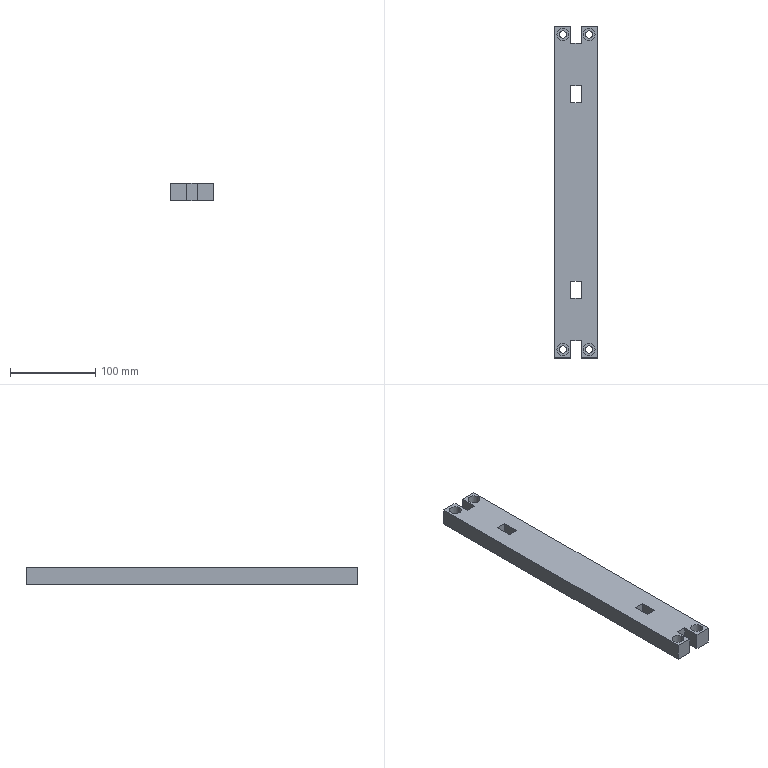Part | STEP file | 冲床-300配套压波_id178_x_t | 1 solid | 34 faces | box 50 x 390 x 20 mm | volume 362265 mm3 | plane 26 | cylinder 8 | commonest cylinder face diameters 8.7 x4 14 x4
STEP:
#1=CARTESIAN_POINT('',(1118.85,-185.,60.));
#2=VERTEX_POINT('',#1);
#3=CARTESIAN_POINT('',(1114.5,-185.,60.));
#4=DIRECTION('',(0.,0.,1.));
#5=DIRECTION('',(1.,0.,0.));
#6=AXIS2_PLACEMENT_3D('',#3,#4,#5);
#7=CIRCLE('',#6,4.35);
#8=EDGE_CURVE('',#2,#2,#7,.T.);
#9=ORIENTED_EDGE('',*,*,#8,.F.);
#10=EDGE_LOOP('',(#9));
#11=FACE_BOUND('',#10,.T.);
#12=CARTESIAN_POINT('',(1121.5,-185.,60.));
#13=VERTEX_POINT('',#12);
#14=CARTESIAN_POINT('',(1114.5,-185.,60.));
#15=DIRECTION('',(0.,0.,1.));
#16=DIRECTION('',(1.,0.,0.));
#17=AXIS2_PLACEMENT_3D('',#14,#15,#16);
#18=CIRCLE('',#17,7.);
#19=EDGE_CURVE('',#13,#13,#18,.T.);
#20=ORIENTED_EDGE('',*,*,#19,.T.);
#21=EDGE_LOOP('',(#20));
#22=FACE_BOUND('',#21,.T.);
#23=CARTESIAN_POINT('',(1114.5,-185.,60.));
#24=DIRECTION('',(0.,0.,-1.));
#25=DIRECTION('',(1.,0.,0.));
#26=AXIS2_PLACEMENT_3D('',#23,#24,#25);
#27=PLANE('',#26);
#28=ADVANCED_FACE('',(#11,#22),#27,.F.);
#29=CARTESIAN_POINT('',(1118.85,-185.,50.));
#30=VERTEX_POINT('',#29);
#31=CARTESIAN_POINT('',(1114.5,-185.,50.));
#32=DIRECTION('',(0.,0.,-1.));
#33=DIRECTION('',(1.,0.,0.));
#34=AXIS2_PLACEMENT_3D('',#31,#32,#33);
#35=CIRCLE('',#34,4.35);
#36=EDGE_CURVE('',#30,#30,#35,.T.);
#37=ORIENTED_EDGE('',*,*,#36,.T.);
#38=EDGE_LOOP('',(#37));
#39=FACE_BOUND('',#38,.T.);
#40=ORIENTED_EDGE('',*,*,#8,.T.);
#41=EDGE_LOOP('',(#40));
#42=FACE_BOUND('',#41,.T.);
#43=CARTESIAN_POINT('',(1114.5,-185.,-46.884));
#44=DIRECTION('',(0.,0.,-1.));
#45=DIRECTION('',(1.,0.,0.));
#46=AXIS2_PLACEMENT_3D('',#43,#44,#45);
#47=CYLINDRICAL_SURFACE('',#46,4.35);
#48=ADVANCED_FACE('',(#39,#42),#47,.F.);
#49=ORIENTED_EDGE('',*,*,#19,.F.);
#50=EDGE_LOOP('',(#49));
#51=FACE_BOUND('',#50,.T.);
#52=CARTESIAN_POINT('',(1121.5,-185.,70.));
#53=VERTEX_POINT('',#52);
#54=CARTESIAN_POINT('',(1114.5,-185.,70.));
#55=DIRECTION('',(0.,0.,1.));
#56=DIRECTION('',(1.,0.,0.));
#57=AXIS2_PLACEMENT_3D('',#54,#55,#56);
#58=CIRCLE('',#57,7.);
#59=EDGE_CURVE('',#53,#53,#58,.T.);
#60=ORIENTED_EDGE('',*,*,#59,.T.);
#61=EDGE_LOOP('',(#60));
#62=FACE_BOUND('',#61,.T.);
#63=CARTESIAN_POINT('',(1114.5,-185.,70.));
#64=DIRECTION('',(0.,0.,-1.));
#65=DIRECTION('',(1.,0.,0.));
#66=AXIS2_PLACEMENT_3D('',#63,#64,#65);
#67=CYLINDRICAL_SURFACE('',#66,7.);
#68=ADVANCED_FACE('',(#51,#62),#67,.F.);
#69=CARTESIAN_POINT('',(1141.15,-185.,60.));
#70=VERTEX_POINT('',#69);
#71=CARTESIAN_POINT('',(1145.5,-185.,60.));
#72=DIRECTION('',(0.,0.,1.));
#73=DIRECTION('',(-1.,0.,0.));
#74=AXIS2_PLACEMENT_3D('',#71,#72,#73);
#75=CIRCLE('',#74,4.35);
#76=EDGE_CURVE('',#70,#70,#75,.T.);
#77=ORIENTED_EDGE('',*,*,#76,.F.);
#78=EDGE_LOOP('',(#77));
#79=FACE_BOUND('',#78,.T.);
#80=CARTESIAN_POINT('',(1138.5,-185.,60.));
#81=VERTEX_POINT('',#80);
#82=CARTESIAN_POINT('',(1145.5,-185.,60.));
#83=DIRECTION('',(0.,0.,1.));
#84=DIRECTION('',(-1.,0.,0.));
#85=AXIS2_PLACEMENT_3D('',#82,#83,#84);
#86=CIRCLE('',#85,7.);
#87=EDGE_CURVE('',#81,#81,#86,.T.);
#88=ORIENTED_EDGE('',*,*,#87,.T.);
#89=EDGE_LOOP('',(#88));
#90=FACE_BOUND('',#89,.T.);
#91=CARTESIAN_POINT('',(1145.5,-185.,60.));
#92=DIRECTION('',(0.,0.,-1.));
#93=DIRECTION('',(-1.,0.,0.));
#94=AXIS2_PLACEMENT_3D('',#91,#92,#93);
#95=PLANE('',#94);
#96=ADVANCED_FACE('',(#79,#90),#95,.F.);
#97=CARTESIAN_POINT('',(1136.,-105.,70.));
#98=VERTEX_POINT('',#97);
#99=CARTESIAN_POINT('',(1136.,-125.,70.));
#100=VERTEX_POINT('',#99);
#101=CARTESIAN_POINT('',(1136.,-105.,70.));
#102=DIRECTION('',(0.,-1.,0.));
#103=VECTOR('',#102,1.);
#104=LINE('',#101,#103);
#105=EDGE_CURVE('',#98,#100,#104,.T.);
#106=ORIENTED_EDGE('',*,*,#105,.F.);
#107=CARTESIAN_POINT('',(1136.,-105.,50.));
#108=VERTEX_POINT('',#107);
#109=CARTESIAN_POINT('',(1136.,-105.,150.));
#110=DIRECTION('',(0.,0.,1.));
#111=VECTOR('',#110,1.);
#112=LINE('',#109,#111);
#113=EDGE_CURVE('',#108,#98,#112,.T.);
#114=ORIENTED_EDGE('',*,*,#113,.F.);
#115=CARTESIAN_POINT('',(1136.,-125.,50.));
#116=VERTEX_POINT('',#115);
#117=CARTESIAN_POINT('',(1136.,-125.,50.));
#118=DIRECTION('',(0.,-1.,0.));
#119=VECTOR('',#118,1.);
#120=LINE('',#117,#119);
#121=EDGE_CURVE('',#108,#116,#120,.T.);
#122=ORIENTED_EDGE('',*,*,#121,.T.);
#123=CARTESIAN_POINT('',(1136.,-125.,46.));
#124=DIRECTION('',(0.,0.,-1.));
#125=VECTOR('',#124,1.);
#126=LINE('',#123,#125);
#127=EDGE_CURVE('',#100,#116,#126,.T.);
#128=ORIENTED_EDGE('',*,*,#127,.F.);
#129=EDGE_LOOP('',(#106,#114,#122,#128));
#130=FACE_OUTER_BOUND('',#129,.T.);
#131=CARTESIAN_POINT('',(1136.,-125.,46.));
#132=DIRECTION('',(1.,0.,0.));
#133=DIRECTION('',(0.,0.,-1.));
#134=AXIS2_PLACEMENT_3D('',#131,#132,#133);
#135=PLANE('',#134);
#136=ADVANCED_FACE('',(#130),#135,.F.);
#137=ORIENTED_EDGE('',*,*,#113,.T.);
#138=CARTESIAN_POINT('',(1124.,-105.,70.));
#139=VERTEX_POINT('',#138);
#140=CARTESIAN_POINT('',(1105.,-105.,70.));
#141=DIRECTION('',(-1.,0.,0.));
#142=VECTOR('',#141,1.);
#143=LINE('',#140,#142);
#144=EDGE_CURVE('',#98,#139,#143,.T.);
#145=ORIENTED_EDGE('',*,*,#144,.T.);
#146=CARTESIAN_POINT('',(1124.,-105.,50.));
#147=VERTEX_POINT('',#146);
#148=CARTESIAN_POINT('',(1124.,-105.,150.));
#149=DIRECTION('',(0.,0.,-1.));
#150=VECTOR('',#149,1.);
#151=LINE('',#148,#150);
#152=EDGE_CURVE('',#139,#147,#151,.T.);
#153=ORIENTED_EDGE('',*,*,#152,.T.);
#154=CARTESIAN_POINT('',(1105.,-105.,50.));
#155=DIRECTION('',(-1.,0.,0.));
#156=VECTOR('',#155,1.);
#157=LINE('',#154,#156);
#158=EDGE_CURVE('',#108,#147,#157,.T.);
#159=ORIENTED_EDGE('',*,*,#158,.F.);
#160=EDGE_LOOP('',(#137,#145,#153,#159));
#161=FACE_OUTER_BOUND('',#160,.T.);
#162=CARTESIAN_POINT('',(1105.,-105.,150.));
#163=DIRECTION('',(0.,-1.,0.));
#164=DIRECTION('',(0.,0.,1.));
#165=AXIS2_PLACEMENT_3D('',#162,#163,#164);
#166=PLANE('',#165);
#167=ADVANCED_FACE('',(#161),#166,.T.);
#168=ORIENTED_EDGE('',*,*,#152,.F.);
#169=CARTESIAN_POINT('',(1124.,-125.,70.));
#170=VERTEX_POINT('',#169);
#171=CARTESIAN_POINT('',(1124.,-105.,70.));
#172=DIRECTION('',(0.,1.,0.));
#173=VECTOR('',#172,1.);
#174=LINE('',#171,#173);
#175=EDGE_CURVE('',#170,#139,#174,.T.);
#176=ORIENTED_EDGE('',*,*,#175,.F.);
#177=CARTESIAN_POINT('',(1124.,-125.,50.));
#178=VERTEX_POINT('',#177);
#179=CARTESIAN_POINT('',(1124.,-125.,78.));
#180=DIRECTION('',(0.,0.,1.));
#181=VECTOR('',#180,1.);
#182=LINE('',#179,#181);
#183=EDGE_CURVE('',#178,#170,#182,.T.);
#184=ORIENTED_EDGE('',*,*,#183,.F.);
#185=CARTESIAN_POINT('',(1124.,-105.,50.));
#186=DIRECTION('',(0.,-1.,0.));
#187=VECTOR('',#186,1.);
#188=LINE('',#185,#187);
#189=EDGE_CURVE('',#147,#178,#188,.T.);
#190=ORIENTED_EDGE('',*,*,#189,.F.);
#191=EDGE_LOOP('',(#168,#176,#184,#190));
#192=FACE_OUTER_BOUND('',#191,.T.);
#193=CARTESIAN_POINT('',(1124.,-125.,78.));
#194=DIRECTION('',(-1.,0.,0.));
#195=DIRECTION('',(0.,0.,1.));
#196=AXIS2_PLACEMENT_3D('',#193,#194,#195);
#197=PLANE('',#196);
#198=ADVANCED_FACE('',(#192),#197,.F.);
#199=ORIENTED_EDGE('',*,*,#183,.T.);
#200=CARTESIAN_POINT('',(1105.,-125.,70.));
#201=DIRECTION('',(1.,0.,0.));
#202=VECTOR('',#201,1.);
#203=LINE('',#200,#202);
#204=EDGE_CURVE('',#170,#100,#203,.T.);
#205=ORIENTED_EDGE('',*,*,#204,.T.);
#206=ORIENTED_EDGE('',*,*,#127,.T.);
#207=CARTESIAN_POINT('',(1155.,-125.,50.));
#208=DIRECTION('',(-1.,0.,0.));
#209=VECTOR('',#208,1.);
#210=LINE('',#207,#209);
#211=EDGE_CURVE('',#116,#178,#210,.T.);
#212=ORIENTED_EDGE('',*,*,#211,.T.);
#213=EDGE_LOOP('',(#199,#205,#206,#212));
#214=FACE_OUTER_BOUND('',#213,.T.);
#215=CARTESIAN_POINT('',(1155.,-125.,150.));
#216=DIRECTION('',(0.,1.,0.));
#217=DIRECTION('',(0.,0.,-1.));
#218=AXIS2_PLACEMENT_3D('',#215,#216,#217);
#219=PLANE('',#218);
#220=ADVANCED_FACE('',(#214),#219,.T.);
#221=CARTESIAN_POINT('',(1155.,-195.,50.));
#222=VERTEX_POINT('',#221);
#223=CARTESIAN_POINT('',(1155.,195.,50.));
#224=VERTEX_POINT('',#223);
#225=CARTESIAN_POINT('',(1155.,-105.,50.));
#226=DIRECTION('',(0.,1.,0.));
#227=VECTOR('',#226,1.);
#228=LINE('',#225,#227);
#229=EDGE_CURVE('',#222,#224,#228,.T.);
#230=ORIENTED_EDGE('',*,*,#229,.T.);
#231=CARTESIAN_POINT('',(1155.,195.,70.));
#232=VERTEX_POINT('',#231);
#233=CARTESIAN_POINT('',(1155.,195.,50.));
#234=DIRECTION('',(0.,0.,-1.));
#235=VECTOR('',#234,1.);
#236=LINE('',#233,#235);
#237=EDGE_CURVE('',#232,#224,#236,.T.);
#238=ORIENTED_EDGE('',*,*,#237,.F.);
#239=CARTESIAN_POINT('',(1155.,-195.,70.));
#240=VERTEX_POINT('',#239);
#241=CARTESIAN_POINT('',(1155.,-105.,70.));
#242=DIRECTION('',(0.,1.,0.));
#243=VECTOR('',#242,1.);
#244=LINE('',#241,#243);
#245=EDGE_CURVE('',#240,#232,#244,.T.);
#246=ORIENTED_EDGE('',*,*,#245,.F.);
#247=CARTESIAN_POINT('',(1155.,-195.,50.));
#248=DIRECTION('',(0.,0.,-1.));
#249=VECTOR('',#248,1.);
#250=LINE('',#247,#249);
#251=EDGE_CURVE('',#240,#222,#250,.T.);
#252=ORIENTED_EDGE('',*,*,#251,.T.);
#253=EDGE_LOOP('',(#230,#238,#246,#252));
#254=FACE_OUTER_BOUND('',#253,.T.);
#255=CARTESIAN_POINT('',(1155.,-105.,70.));
#256=DIRECTION('',(1.,0.,0.));
#257=DIRECTION('',(0.,0.,-1.));
#258=AXIS2_PLACEMENT_3D('',#255,#256,#257);
#259=PLANE('',#258);
#260=ADVANCED_FACE('',(#254),#259,.T.);
#261=CARTESIAN_POINT('',(1136.,-195.,50.));
#262=VERTEX_POINT('',#261);
#263=CARTESIAN_POINT('',(1136.,-195.,70.));
#264=VERTEX_POINT('',#263);
#265=CARTESIAN_POINT('',(1136.,-195.,70.));
#266=DIRECTION('',(0.,0.,1.));
#267=VECTOR('',#266,1.);
#268=LINE('',#265,#267);
#269=EDGE_CURVE('',#262,#264,#268,.T.);
#270=ORIENTED_EDGE('',*,*,#269,.F.);
#271=CARTESIAN_POINT('',(1155.,-195.,50.));
#272=DIRECTION('',(-1.,0.,0.));
#273=VECTOR('',#272,1.);
#274=LINE('',#271,#273);
#275=EDGE_CURVE('',#222,#262,#274,.T.);
#276=ORIENTED_EDGE('',*,*,#275,.F.);
#277=ORIENTED_EDGE('',*,*,#251,.F.);
#278=CARTESIAN_POINT('',(1155.,-195.,70.));
#279=DIRECTION('',(1.,0.,0.));
#280=VECTOR('',#279,1.);
#281=LINE('',#278,#280);
#282=EDGE_CURVE('',#264,#240,#281,.T.);
#283=ORIENTED_EDGE('',*,*,#282,.F.);
#284=EDGE_LOOP('',(#270,#276,#277,#283));
#285=FACE_OUTER_BOUND('',#284,.T.);
#286=CARTESIAN_POINT('',(1155.,-195.,50.));
#287=DIRECTION('',(0.,1.,0.));
#288=DIRECTION('',(0.,0.,-1.));
#289=AXIS2_PLACEMENT_3D('',#286,#287,#288);
#290=PLANE('',#289);
#291=ADVANCED_FACE('',(#285),#290,.F.);
#292=ORIENTED_EDGE('',*,*,#269,.T.);
#293=CARTESIAN_POINT('',(1136.,-175.,70.));
#294=VERTEX_POINT('',#293);
#295=CARTESIAN_POINT('',(1136.,-175.,70.));
#296=DIRECTION('',(0.,-1.,0.));
#297=VECTOR('',#296,1.);
#298=LINE('',#295,#297);
#299=EDGE_CURVE('',#294,#264,#298,.T.);
#300=ORIENTED_EDGE('',*,*,#299,.F.);
#301=CARTESIAN_POINT('',(1136.,-175.,50.));
#302=VERTEX_POINT('',#301);
#303=CARTESIAN_POINT('',(1136.,-175.,70.));
#304=DIRECTION('',(0.,0.,-1.));
#305=VECTOR('',#304,1.);
#306=LINE('',#303,#305);
#307=EDGE_CURVE('',#294,#302,#306,.T.);
#308=ORIENTED_EDGE('',*,*,#307,.T.);
#309=CARTESIAN_POINT('',(1136.,-175.,50.));
#310=DIRECTION('',(0.,-1.,0.));
#311=VECTOR('',#310,1.);
#312=LINE('',#309,#311);
#313=EDGE_CURVE('',#302,#262,#312,.T.);
#314=ORIENTED_EDGE('',*,*,#313,.T.);
#315=EDGE_LOOP('',(#292,#300,#308,#314));
#316=FACE_OUTER_BOUND('',#315,.T.);
#317=CARTESIAN_POINT('',(1136.,-175.,70.));
#318=DIRECTION('',(1.,0.,0.));
#319=DIRECTION('',(0.,0.,-1.));
#320=AXIS2_PLACEMENT_3D('',#317,#318,#319);
#321=PLANE('',#320);
#322=ADVANCED_FACE('',(#316),#321,.F.);
#323=CARTESIAN_POINT('',(1124.,-175.,50.));
#324=VERTEX_POINT('',#323);
#325=CARTESIAN_POINT('',(1155.,-175.,50.));
#326=DIRECTION('',(-1.,0.,0.));
#327=VECTOR('',#326,1.);
#328=LINE('',#325,#327);
#329=EDGE_CURVE('',#302,#324,#328,.T.);
#330=ORIENTED_EDGE('',*,*,#329,.F.);
#331=ORIENTED_EDGE('',*,*,#307,.F.);
#332=CARTESIAN_POINT('',(1124.,-175.,70.));
#333=VERTEX_POINT('',#332);
#334=CARTESIAN_POINT('',(1124.,-175.,70.));
#335=DIRECTION('',(1.,0.,0.));
#336=VECTOR('',#335,1.);
#337=LINE('',#334,#336);
#338=EDGE_CURVE('',#333,#294,#337,.T.);
#339=ORIENTED_EDGE('',*,*,#338,.F.);
#340=CARTESIAN_POINT('',(1124.,-175.,50.));
#341=DIRECTION('',(0.,0.,1.));
#342=VECTOR('',#341,1.);
#343=LINE('',#340,#342);
#344=EDGE_CURVE('',#324,#333,#343,.T.);
#345=ORIENTED_EDGE('',*,*,#344,.F.);
#346=EDGE_LOOP('',(#330,#331,#339,#345));
#347=FACE_OUTER_BOUND('',#346,.T.);
#348=CARTESIAN_POINT('',(1155.,-175.,50.));
#349=DIRECTION('',(0.,1.,0.));
#350=DIRECTION('',(0.,0.,-1.));
#351=AXIS2_PLACEMENT_3D('',#348,#349,#350);
#352=PLANE('',#351);
#353=ADVANCED_FACE('',(#347),#352,.F.);
#354=CARTESIAN_POINT('',(1124.,-195.,70.));
#355=VERTEX_POINT('',#354);
#356=CARTESIAN_POINT('',(1124.,-195.,50.));
#357=VERTEX_POINT('',#356);
#358=CARTESIAN_POINT('',(1124.,-195.,50.));
#359=DIRECTION('',(0.,0.,-1.));
#360=VECTOR('',#359,1.);
#361=LINE('',#358,#360);
#362=EDGE_CURVE('',#355,#357,#361,.T.);
#363=ORIENTED_EDGE('',*,*,#362,.T.);
#364=CARTESIAN_POINT('',(1124.,-175.,50.));
#365=DIRECTION('',(0.,-1.,0.));
#366=VECTOR('',#365,1.);
#367=LINE('',#364,#366);
#368=EDGE_CURVE('',#324,#357,#367,.T.);
#369=ORIENTED_EDGE('',*,*,#368,.F.);
#370=ORIENTED_EDGE('',*,*,#344,.T.);
#371=CARTESIAN_POINT('',(1124.,-175.,70.));
#372=DIRECTION('',(0.,-1.,0.));
#373=VECTOR('',#372,1.);
#374=LINE('',#371,#373);
#375=EDGE_CURVE('',#333,#355,#374,.T.);
#376=ORIENTED_EDGE('',*,*,#375,.T.);
#377=EDGE_LOOP('',(#363,#369,#370,#376));
#378=FACE_OUTER_BOUND('',#377,.T.);
#379=CARTESIAN_POINT('',(1124.,-175.,50.));
#380=DIRECTION('',(-1.,0.,0.));
#381=DIRECTION('',(0.,0.,1.));
#382=AXIS2_PLACEMENT_3D('',#379,#380,#381);
#383=PLANE('',#382);
#384=ADVANCED_FACE('',(#378),#383,.F.);
#385=ORIENTED_EDGE('',*,*,#362,.F.);
#386=CARTESIAN_POINT('',(1105.,-195.,70.));
#387=VERTEX_POINT('',#386);
#388=CARTESIAN_POINT('',(1155.,-195.,70.));
#389=DIRECTION('',(1.,0.,0.));
#390=VECTOR('',#389,1.);
#391=LINE('',#388,#390);
#392=EDGE_CURVE('',#387,#355,#391,.T.);
#393=ORIENTED_EDGE('',*,*,#392,.F.);
#394=CARTESIAN_POINT('',(1105.,-195.,50.));
#395=VERTEX_POINT('',#394);
#396=CARTESIAN_POINT('',(1105.,-195.,50.));
#397=DIRECTION('',(0.,0.,1.));
#398=VECTOR('',#397,1.);
#399=LINE('',#396,#398);
#400=EDGE_CURVE('',#395,#387,#399,.T.);
#401=ORIENTED_EDGE('',*,*,#400,.F.);
#402=CARTESIAN_POINT('',(1155.,-195.,50.));
#403=DIRECTION('',(-1.,0.,0.));
#404=VECTOR('',#403,1.);
#405=LINE('',#402,#404);
#406=EDGE_CURVE('',#357,#395,#405,.T.);
#407=ORIENTED_EDGE('',*,*,#406,.F.);
#408=EDGE_LOOP('',(#385,#393,#401,#407));
#409=FACE_OUTER_BOUND('',#408,.T.);
#410=CARTESIAN_POINT('',(1155.,-195.,50.));
#411=DIRECTION('',(0.,1.,0.));
#412=DIRECTION('',(0.,0.,-1.));
#413=AXIS2_PLACEMENT_3D('',#410,#411,#412);
#414=PLANE('',#413);
#415=ADVANCED_FACE('',(#409),#414,.F.);
#416=CARTESIAN_POINT('',(1105.,195.,70.));
#417=VERTEX_POINT('',#416);
#418=CARTESIAN_POINT('',(1105.,-105.,70.));
#419=DIRECTION('',(0.,1.,0.));
#420=VECTOR('',#419,1.);
#421=LINE('',#418,#420);
#422=EDGE_CURVE('',#387,#417,#421,.T.);
#423=ORIENTED_EDGE('',*,*,#422,.T.);
#424=CARTESIAN_POINT('',(1105.,195.,50.));
#425=VERTEX_POINT('',#424);
#426=CARTESIAN_POINT('',(1105.,195.,50.));
#427=DIRECTION('',(0.,0.,1.));
#428=VECTOR('',#427,1.);
#429=LINE('',#426,#428);
#430=EDGE_CURVE('',#425,#417,#429,.T.);
#431=ORIENTED_EDGE('',*,*,#430,.F.);
#432=CARTESIAN_POINT('',(1105.,-105.,50.));
#433=DIRECTION('',(0.,1.,0.));
#434=VECTOR('',#433,1.);
#435=LINE('',#432,#434);
#436=EDGE_CURVE('',#395,#425,#435,.T.);
#437=ORIENTED_EDGE('',*,*,#436,.F.);
#438=ORIENTED_EDGE('',*,*,#400,.T.);
#439=EDGE_LOOP('',(#423,#431,#437,#438));
#440=FACE_OUTER_BOUND('',#439,.T.);
#441=CARTESIAN_POINT('',(1105.,-105.,50.));
#442=DIRECTION('',(-1.,0.,0.));
#443=DIRECTION('',(0.,0.,1.));
#444=AXIS2_PLACEMENT_3D('',#441,#442,#443);
#445=PLANE('',#444);
#446=ADVANCED_FACE('',(#440),#445,.T.);
#447=CARTESIAN_POINT('',(1141.15,-185.,50.));
#448=VERTEX_POINT('',#447);
#449=CARTESIAN_POINT('',(1145.5,-185.,50.));
#450=DIRECTION('',(0.,0.,1.));
#451=DIRECTION('',(-1.,0.,0.));
#452=AXIS2_PLACEMENT_3D('',#449,#450,#451);
#453=CIRCLE('',#452,4.35);
#454=EDGE_CURVE('',#448,#448,#453,.T.);
#455=ORIENTED_EDGE('',*,*,#454,.F.);
#456=EDGE_LOOP('',(#455));
#457=FACE_BOUND('',#456,.T.);
#458=ORIENTED_EDGE('',*,*,#76,.T.);
#459=EDGE_LOOP('',(#458));
#460=FACE_BOUND('',#459,.T.);
#461=CARTESIAN_POINT('',(1145.5,-185.,-46.884));
#462=DIRECTION('',(0.,0.,-1.));
#463=DIRECTION('',(-1.,0.,0.));
#464=AXIS2_PLACEMENT_3D('',#461,#462,#463);
#465=CYLINDRICAL_SURFACE('',#464,4.35);
#466=ADVANCED_FACE('',(#457,#460),#465,.F.);
#467=ORIENTED_EDGE('',*,*,#436,.T.);
#468=CARTESIAN_POINT('',(1124.,195.,50.));
#469=VERTEX_POINT('',#468);
#470=CARTESIAN_POINT('',(1155.,195.,50.));
#471=DIRECTION('',(-1.,0.,0.));
#472=VECTOR('',#471,1.);
#473=LINE('',#470,#472);
#474=EDGE_CURVE('',#469,#425,#473,.T.);
#475=ORIENTED_EDGE('',*,*,#474,.F.);
#476=CARTESIAN_POINT('',(1124.,175.,50.));
#477=VERTEX_POINT('',#476);
#478=CARTESIAN_POINT('',(1124.,175.,50.));
#479=DIRECTION('',(0.,1.,0.));
#480=VECTOR('',#479,1.);
#481=LINE('',#478,#480);
#482=EDGE_CURVE('',#477,#469,#481,.T.);
#483=ORIENTED_EDGE('',*,*,#482,.F.);
#484=CARTESIAN_POINT('',(1136.,175.,50.));
#485=VERTEX_POINT('',#484);
#486=CARTESIAN_POINT('',(1155.,175.,50.));
#487=DIRECTION('',(-1.,0.,0.));
#488=VECTOR('',#487,1.);
#489=LINE('',#486,#488);
#490=EDGE_CURVE('',#485,#477,#489,.T.);
#491=ORIENTED_EDGE('',*,*,#490,.F.);
#492=CARTESIAN_POINT('',(1136.,195.,50.));
#493=VERTEX_POINT('',#492);
#494=CARTESIAN_POINT('',(1136.,175.,50.));
#495=DIRECTION('',(0.,1.,0.));
#496=VECTOR('',#495,1.);
#497=LINE('',#494,#496);
#498=EDGE_CURVE('',#485,#493,#497,.T.);
#499=ORIENTED_EDGE('',*,*,#498,.T.);
#500=CARTESIAN_POINT('',(1155.,195.,50.));
#501=DIRECTION('',(-1.,0.,0.));
#502=VECTOR('',#501,1.);
#503=LINE('',#500,#502);
#504=EDGE_CURVE('',#224,#493,#503,.T.);
#505=ORIENTED_EDGE('',*,*,#504,.F.);
#506=ORIENTED_EDGE('',*,*,#229,.F.);
#507=ORIENTED_EDGE('',*,*,#275,.T.);
#508=ORIENTED_EDGE('',*,*,#313,.F.);
#509=ORIENTED_EDGE('',*,*,#329,.T.);
#510=ORIENTED_EDGE('',*,*,#368,.T.);
#511=ORIENTED_EDGE('',*,*,#406,.T.);
#512=EDGE_LOOP('',(#467,#475,#483,#491,#499,#505,#506,#507,#508,#509,#510,#511));
#513=FACE_BOUND('',#512,.T.);
#514=ORIENTED_EDGE('',*,*,#36,.F.);
#515=EDGE_LOOP('',(#514));
#516=FACE_BOUND('',#515,.T.);
#517=ORIENTED_EDGE('',*,*,#454,.T.);
#518=EDGE_LOOP('',(#517));
#519=FACE_BOUND('',#518,.T.);
#520=ORIENTED_EDGE('',*,*,#211,.F.);
#521=ORIENTED_EDGE('',*,*,#121,.F.);
#522=ORIENTED_EDGE('',*,*,#158,.T.);
#523=ORIENTED_EDGE('',*,*,#189,.T.);
#524=EDGE_LOOP('',(#520,#521,#522,#523));
#525=FACE_BOUND('',#524,.T.);
#526=CARTESIAN_POINT('',(1118.85,185.,50.));
#527=VERTEX_POINT('',#526);
#528=CARTESIAN_POINT('',(1114.5,185.,50.));
#529=DIRECTION('',(0.,0.,1.));
#530=DIRECTION('',(1.,0.,0.));
#531=AXIS2_PLACEMENT_3D('',#528,#529,#530);
#532=CIRCLE('',#531,4.35);
#533=EDGE_CURVE('',#527,#527,#532,.T.);
#534=ORIENTED_EDGE('',*,*,#533,.T.);
#535=EDGE_LOOP('',(#534));
#536=FACE_BOUND('',#535,.T.);
#537=CARTESIAN_POINT('',(1141.15,185.,50.));
#538=VERTEX_POINT('',#537);
#539=CARTESIAN_POINT('',(1145.5,185.,50.));
#540=DIRECTION('',(0.,0.,-1.));
#541=DIRECTION('',(-1.,0.,0.));
#542=AXIS2_PLACEMENT_3D('',#539,#540,#541);
#543=CIRCLE('',#542,4.35);
#544=EDGE_CURVE('',#538,#538,#543,.T.);
#545=ORIENTED_EDGE('',*,*,#544,.F.);
#546=EDGE_LOOP('',(#545));
#547=FACE_BOUND('',#546,.T.);
#548=CARTESIAN_POINT('',(1136.,125.,50.));
#549=VERTEX_POINT('',#548);
#550=CARTESIAN_POINT('',(1124.,125.,50.));
#551=VERTEX_POINT('',#550);
#552=CARTESIAN_POINT('',(1155.,125.,50.));
#553=DIRECTION('',(-1.,0.,0.));
#554=VECTOR('',#553,1.);
#555=LINE('',#552,#554);
#556=EDGE_CURVE('',#549,#551,#555,.T.);
#557=ORIENTED_EDGE('',*,*,#556,.T.);
#558=CARTESIAN_POINT('',(1124.,105.,50.));
#559=VERTEX_POINT('',#558);
#560=CARTESIAN_POINT('',(1124.,105.,50.));
#561=DIRECTION('',(0.,1.,0.));
#562=VECTOR('',#561,1.);
#563=LINE('',#560,#562);
#564=EDGE_CURVE('',#559,#551,#563,.T.);
#565=ORIENTED_EDGE('',*,*,#564,.F.);
#566=CARTESIAN_POINT('',(1136.,105.,50.));
#567=VERTEX_POINT('',#566);
#568=CARTESIAN_POINT('',(1105.,105.,50.));
#569=DIRECTION('',(-1.,0.,0.));
#570=VECTOR('',#569,1.);
#571=LINE('',#568,#570);
#572=EDGE_CURVE('',#567,#559,#571,.T.);
#573=ORIENTED_EDGE('',*,*,#572,.F.);
#574=CARTESIAN_POINT('',(1136.,125.,50.));
#575=DIRECTION('',(0.,1.,0.));
#576=VECTOR('',#575,1.);
#577=LINE('',#574,#576);
#578=EDGE_CURVE('',#567,#549,#577,.T.);
#579=ORIENTED_EDGE('',*,*,#578,.T.);
#580=EDGE_LOOP('',(#557,#565,#573,#579));
#581=FACE_BOUND('',#580,.T.);
#582=CARTESIAN_POINT('',(1155.,-105.,50.));
#583=DIRECTION('',(0.,0.,-1.));
#584=DIRECTION('',(-1.,0.,0.));
#585=AXIS2_PLACEMENT_3D('',#582,#583,#584);
#586=PLANE('',#585);
#587=ADVANCED_FACE('',(#513,#516,#519,#525,#536,#547,#581),#586,.T.);
#588=ORIENTED_EDGE('',*,*,#87,.F.);
#589=EDGE_LOOP('',(#588));
#590=FACE_BOUND('',#589,.T.);
#591=CARTESIAN_POINT('',(1138.5,-185.,70.));
#592=VERTEX_POINT('',#591);
#593=CARTESIAN_POINT('',(1145.5,-185.,70.));
#594=DIRECTION('',(0.,0.,1.));
#595=DIRECTION('',(-1.,0.,0.));
#596=AXIS2_PLACEMENT_3D('',#593,#594,#595);
#597=CIRCLE('',#596,7.);
#598=EDGE_CURVE('',#592,#592,#597,.T.);
#599=ORIENTED_EDGE('',*,*,#598,.T.);
#600=EDGE_LOOP('',(#599));
#601=FACE_BOUND('',#600,.T.);
#602=CARTESIAN_POINT('',(1145.5,-185.,70.));
#603=DIRECTION('',(0.,0.,-1.));
#604=DIRECTION('',(-1.,0.,0.));
#605=AXIS2_PLACEMENT_3D('',#602,#603,#604);
#606=CYLINDRICAL_SURFACE('',#605,7.);
#607=ADVANCED_FACE('',(#590,#601),#606,.F.);
#608=ORIENTED_EDGE('',*,*,#245,.T.);
#609=CARTESIAN_POINT('',(1136.,195.,70.));
#610=VERTEX_POINT('',#609);
#611=CARTESIAN_POINT('',(1155.,195.,70.));
#612=DIRECTION('',(1.,0.,0.));
#613=VECTOR('',#612,1.);
#614=LINE('',#611,#613);
#615=EDGE_CURVE('',#610,#232,#614,.T.);
#616=ORIENTED_EDGE('',*,*,#615,.F.);
#617=CARTESIAN_POINT('',(1136.,175.,70.));
#618=VERTEX_POINT('',#617);
#619=CARTESIAN_POINT('',(1136.,175.,70.));
#620=DIRECTION('',(0.,1.,0.));
#621=VECTOR('',#620,1.);
#622=LINE('',#619,#621);
#623=EDGE_CURVE('',#618,#610,#622,.T.);
#624=ORIENTED_EDGE('',*,*,#623,.F.);
#625=CARTESIAN_POINT('',(1124.,175.,70.));
#626=VERTEX_POINT('',#625);
#627=CARTESIAN_POINT('',(1124.,175.,70.));
#628=DIRECTION('',(1.,0.,0.));
#629=VECTOR('',#628,1.);
#630=LINE('',#627,#629);
#631=EDGE_CURVE('',#626,#618,#630,.T.);
#632=ORIENTED_EDGE('',*,*,#631,.F.);
#633=CARTESIAN_POINT('',(1124.,195.,70.));
#634=VERTEX_POINT('',#633);
#635=CARTESIAN_POINT('',(1124.,175.,70.));
#636=DIRECTION('',(0.,1.,0.));
#637=VECTOR('',#636,1.);
#638=LINE('',#635,#637);
#639=EDGE_CURVE('',#626,#634,#638,.T.);
#640=ORIENTED_EDGE('',*,*,#639,.T.);
#641=CARTESIAN_POINT('',(1155.,195.,70.));
#642=DIRECTION('',(1.,0.,0.));
#643=VECTOR('',#642,1.);
#644=LINE('',#641,#643);
#645=EDGE_CURVE('',#417,#634,#644,.T.);
#646=ORIENTED_EDGE('',*,*,#645,.F.);
#647=ORIENTED_EDGE('',*,*,#422,.F.);
#648=ORIENTED_EDGE('',*,*,#392,.T.);
#649=ORIENTED_EDGE('',*,*,#375,.F.);
#650=ORIENTED_EDGE('',*,*,#338,.T.);
#651=ORIENTED_EDGE('',*,*,#299,.T.);
#652=ORIENTED_EDGE('',*,*,#282,.T.);
#653=EDGE_LOOP('',(#608,#616,#624,#632,#640,#646,#647,#648,#649,#650,#651,#652));
#654=FACE_BOUND('',#653,.T.);
#655=ORIENTED_EDGE('',*,*,#59,.F.);
#656=EDGE_LOOP('',(#655));
#657=FACE_BOUND('',#656,.T.);
#658=ORIENTED_EDGE('',*,*,#598,.F.);
#659=EDGE_LOOP('',(#658));
#660=FACE_BOUND('',#659,.T.);
#661=ORIENTED_EDGE('',*,*,#204,.F.);
#662=ORIENTED_EDGE('',*,*,#175,.T.);
#663=ORIENTED_EDGE('',*,*,#144,.F.);
#664=ORIENTED_EDGE('',*,*,#105,.T.);
#665=EDGE_LOOP('',(#661,#662,#663,#664));
#666=FACE_BOUND('',#665,.T.);
#667=CARTESIAN_POINT('',(1121.5,185.,70.));
#668=VERTEX_POINT('',#667);
#669=CARTESIAN_POINT('',(1114.5,185.,70.));
#670=DIRECTION('',(0.,0.,-1.));
#671=DIRECTION('',(1.,0.,0.));
#672=AXIS2_PLACEMENT_3D('',#669,#670,#671);
#673=CIRCLE('',#672,7.);
#674=EDGE_CURVE('',#668,#668,#673,.T.);
#675=ORIENTED_EDGE('',*,*,#674,.T.);
#676=EDGE_LOOP('',(#675));
#677=FACE_BOUND('',#676,.T.);
#678=CARTESIAN_POINT('',(1138.5,185.,70.));
#679=VERTEX_POINT('',#678);
#680=CARTESIAN_POINT('',(1145.5,185.,70.));
#681=DIRECTION('',(0.,0.,-1.));
#682=DIRECTION('',(-1.,0.,0.));
#683=AXIS2_PLACEMENT_3D('',#680,#681,#682);
#684=CIRCLE('',#683,7.);
#685=EDGE_CURVE('',#679,#679,#684,.T.);
#686=ORIENTED_EDGE('',*,*,#685,.T.);
#687=EDGE_LOOP('',(#686));
#688=FACE_BOUND('',#687,.T.);
#689=CARTESIAN_POINT('',(1124.,125.,70.));
#690=VERTEX_POINT('',#689);
#691=CARTESIAN_POINT('',(1136.,125.,70.));
#692=VERTEX_POINT('',#691);
#693=CARTESIAN_POINT('',(1105.,125.,70.));
#694=DIRECTION('',(1.,0.,0.));
#695=VECTOR('',#694,1.);
#696=LINE('',#693,#695);
#697=EDGE_CURVE('',#690,#692,#696,.T.);
#698=ORIENTED_EDGE('',*,*,#697,.T.);
#699=CARTESIAN_POINT('',(1136.,105.,70.));
#700=VERTEX_POINT('',#699);
#701=CARTESIAN_POINT('',(1136.,105.,70.));
#702=DIRECTION('',(0.,1.,0.));
#703=VECTOR('',#702,1.);
#704=LINE('',#701,#703);
#705=EDGE_CURVE('',#700,#692,#704,.T.);
#706=ORIENTED_EDGE('',*,*,#705,.F.);
#707=CARTESIAN_POINT('',(1124.,105.,70.));
#708=VERTEX_POINT('',#707);
#709=CARTESIAN_POINT('',(1105.,105.,70.));
#710=DIRECTION('',(-1.,0.,0.));
#711=VECTOR('',#710,1.);
#712=LINE('',#709,#711);
#713=EDGE_CURVE('',#700,#708,#712,.T.);
#714=ORIENTED_EDGE('',*,*,#713,.T.);
#715=CARTESIAN_POINT('',(1124.,105.,70.));
#716=DIRECTION('',(0.,-1.,0.));
#717=VECTOR('',#716,1.);
#718=LINE('',#715,#717);
#719=EDGE_CURVE('',#690,#708,#718,.T.);
#720=ORIENTED_EDGE('',*,*,#719,.F.);
#721=EDGE_LOOP('',(#698,#706,#714,#720));
#722=FACE_BOUND('',#721,.T.);
#723=CARTESIAN_POINT('',(1105.,-105.,70.));
#724=DIRECTION('',(0.,0.,1.));
#725=DIRECTION('',(1.,0.,0.));
#726=AXIS2_PLACEMENT_3D('',#723,#724,#725);
#727=PLANE('',#726);
#728=ADVANCED_FACE('',(#654,#657,#660,#666,#677,#688,#722),#727,.T.);
#729=CARTESIAN_POINT('',(1118.85,185.,60.));
#730=VERTEX_POINT('',#729);
#731=CARTESIAN_POINT('',(1114.5,185.,60.));
#732=DIRECTION('',(0.,0.,1.));
#733=DIRECTION('',(1.,0.,0.));
#734=AXIS2_PLACEMENT_3D('',#731,#732,#733);
#735=CIRCLE('',#734,4.35);
#736=EDGE_CURVE('',#730,#730,#735,.T.);
#737=ORIENTED_EDGE('',*,*,#736,.F.);
#738=EDGE_LOOP('',(#737));
#739=FACE_BOUND('',#738,.T.);
#740=CARTESIAN_POINT('',(1121.5,185.,60.));
#741=VERTEX_POINT('',#740);
#742=CARTESIAN_POINT('',(1114.5,185.,60.));
#743=DIRECTION('',(0.,0.,1.));
#744=DIRECTION('',(1.,0.,0.));
#745=AXIS2_PLACEMENT_3D('',#742,#743,#744);
#746=CIRCLE('',#745,7.);
#747=EDGE_CURVE('',#741,#741,#746,.T.);
#748=ORIENTED_EDGE('',*,*,#747,.T.);
#749=EDGE_LOOP('',(#748));
#750=FACE_BOUND('',#749,.T.);
#751=CARTESIAN_POINT('',(1114.5,185.,60.));
#752=DIRECTION('',(0.,0.,-1.));
#753=DIRECTION('',(1.,0.,0.));
#754=AXIS2_PLACEMENT_3D('',#751,#752,#753);
#755=PLANE('',#754);
#756=ADVANCED_FACE('',(#739,#750),#755,.F.);
#757=ORIENTED_EDGE('',*,*,#533,.F.);
#758=EDGE_LOOP('',(#757));
#759=FACE_BOUND('',#758,.T.);
#760=ORIENTED_EDGE('',*,*,#736,.T.);
#761=EDGE_LOOP('',(#760));
#762=FACE_BOUND('',#761,.T.);
#763=CARTESIAN_POINT('',(1114.5,185.,-46.884));
#764=DIRECTION('',(0.,0.,-1.));
#765=DIRECTION('',(1.,0.,0.));
#766=AXIS2_PLACEMENT_3D('',#763,#764,#765);
#767=CYLINDRICAL_SURFACE('',#766,4.35);
#768=ADVANCED_FACE('',(#759,#762),#767,.F.);
#769=ORIENTED_EDGE('',*,*,#747,.F.);
#770=EDGE_LOOP('',(#769));
#771=FACE_BOUND('',#770,.T.);
#772=ORIENTED_EDGE('',*,*,#674,.F.);
#773=EDGE_LOOP('',(#772));
#774=FACE_BOUND('',#773,.T.);
#775=CARTESIAN_POINT('',(1114.5,185.,70.));
#776=DIRECTION('',(0.,0.,-1.));
#777=DIRECTION('',(1.,0.,0.));
#778=AXIS2_PLACEMENT_3D('',#775,#776,#777);
#779=CYLINDRICAL_SURFACE('',#778,7.);
#780=ADVANCED_FACE('',(#771,#774),#779,.F.);
#781=CARTESIAN_POINT('',(1141.15,185.,60.));
#782=VERTEX_POINT('',#781);
#783=CARTESIAN_POINT('',(1145.5,185.,60.));
#784=DIRECTION('',(0.,0.,1.));
#785=DIRECTION('',(-1.,0.,0.));
#786=AXIS2_PLACEMENT_3D('',#783,#784,#785);
#787=CIRCLE('',#786,4.35);
#788=EDGE_CURVE('',#782,#782,#787,.T.);
#789=ORIENTED_EDGE('',*,*,#788,.F.);
#790=EDGE_LOOP('',(#789));
#791=FACE_BOUND('',#790,.T.);
#792=CARTESIAN_POINT('',(1138.5,185.,60.));
#793=VERTEX_POINT('',#792);
#794=CARTESIAN_POINT('',(1145.5,185.,60.));
#795=DIRECTION('',(0.,0.,1.));
#796=DIRECTION('',(-1.,0.,0.));
#797=AXIS2_PLACEMENT_3D('',#794,#795,#796);
#798=CIRCLE('',#797,7.);
#799=EDGE_CURVE('',#793,#793,#798,.T.);
#800=ORIENTED_EDGE('',*,*,#799,.T.);
#801=EDGE_LOOP('',(#800));
#802=FACE_BOUND('',#801,.T.);
#803=CARTESIAN_POINT('',(1145.5,185.,60.));
#804=DIRECTION('',(0.,0.,-1.));
#805=DIRECTION('',(-1.,0.,0.));
#806=AXIS2_PLACEMENT_3D('',#803,#804,#805);
#807=PLANE('',#806);
#808=ADVANCED_FACE('',(#791,#802),#807,.F.);
#809=ORIENTED_EDGE('',*,*,#705,.T.);
#810=CARTESIAN_POINT('',(1136.,125.,46.));
#811=DIRECTION('',(0.,0.,1.));
#812=VECTOR('',#811,1.);
#813=LINE('',#810,#812);
#814=EDGE_CURVE('',#549,#692,#813,.T.);
#815=ORIENTED_EDGE('',*,*,#814,.F.);
#816=ORIENTED_EDGE('',*,*,#578,.F.);
#817=CARTESIAN_POINT('',(1136.,105.,150.));
#818=DIRECTION('',(0.,0.,-1.));
#819=VECTOR('',#818,1.);
#820=LINE('',#817,#819);
#821=EDGE_CURVE('',#700,#567,#820,.T.);
#822=ORIENTED_EDGE('',*,*,#821,.F.);
#823=EDGE_LOOP('',(#809,#815,#816,#822));
#824=FACE_OUTER_BOUND('',#823,.T.);
#825=CARTESIAN_POINT('',(1136.,125.,46.));
#826=DIRECTION('',(1.,0.,0.));
#827=DIRECTION('',(0.,0.,-1.));
#828=AXIS2_PLACEMENT_3D('',#825,#826,#827);
#829=PLANE('',#828);
#830=ADVANCED_FACE('',(#824),#829,.F.);
#831=ORIENTED_EDGE('',*,*,#821,.T.);
#832=ORIENTED_EDGE('',*,*,#572,.T.);
#833=CARTESIAN_POINT('',(1124.,105.,150.));
#834=DIRECTION('',(0.,0.,1.));
#835=VECTOR('',#834,1.);
#836=LINE('',#833,#835);
#837=EDGE_CURVE('',#559,#708,#836,.T.);
#838=ORIENTED_EDGE('',*,*,#837,.T.);
#839=ORIENTED_EDGE('',*,*,#713,.F.);
#840=EDGE_LOOP('',(#831,#832,#838,#839));
#841=FACE_OUTER_BOUND('',#840,.T.);
#842=CARTESIAN_POINT('',(1105.,105.,150.));
#843=DIRECTION('',(0.,1.,0.));
#844=DIRECTION('',(0.,0.,1.));
#845=AXIS2_PLACEMENT_3D('',#842,#843,#844);
#846=PLANE('',#845);
#847=ADVANCED_FACE('',(#841),#846,.T.);
#848=ORIENTED_EDGE('',*,*,#837,.F.);
#849=ORIENTED_EDGE('',*,*,#564,.T.);
#850=CARTESIAN_POINT('',(1124.,125.,78.));
#851=DIRECTION('',(0.,0.,-1.));
#852=VECTOR('',#851,1.);
#853=LINE('',#850,#852);
#854=EDGE_CURVE('',#690,#551,#853,.T.);
#855=ORIENTED_EDGE('',*,*,#854,.F.);
#856=ORIENTED_EDGE('',*,*,#719,.T.);
#857=EDGE_LOOP('',(#848,#849,#855,#856));
#858=FACE_OUTER_BOUND('',#857,.T.);
#859=CARTESIAN_POINT('',(1124.,125.,78.));
#860=DIRECTION('',(-1.,0.,0.));
#861=DIRECTION('',(0.,0.,1.));
#862=AXIS2_PLACEMENT_3D('',#859,#860,#861);
#863=PLANE('',#862);
#864=ADVANCED_FACE('',(#858),#863,.F.);
#865=ORIENTED_EDGE('',*,*,#854,.T.);
#866=ORIENTED_EDGE('',*,*,#556,.F.);
#867=ORIENTED_EDGE('',*,*,#814,.T.);
#868=ORIENTED_EDGE('',*,*,#697,.F.);
#869=EDGE_LOOP('',(#865,#866,#867,#868));
#870=FACE_OUTER_BOUND('',#869,.T.);
#871=CARTESIAN_POINT('',(1155.,125.,150.));
#872=DIRECTION('',(0.,-1.,0.));
#873=DIRECTION('',(0.,0.,-1.));
#874=AXIS2_PLACEMENT_3D('',#871,#872,#873);
#875=PLANE('',#874);
#876=ADVANCED_FACE('',(#870),#875,.T.);
#877=CARTESIAN_POINT('',(1136.,195.,70.));
#878=DIRECTION('',(0.,0.,-1.));
#879=VECTOR('',#878,1.);
#880=LINE('',#877,#879);
#881=EDGE_CURVE('',#610,#493,#880,.T.);
#882=ORIENTED_EDGE('',*,*,#881,.F.);
#883=ORIENTED_EDGE('',*,*,#615,.T.);
#884=ORIENTED_EDGE('',*,*,#237,.T.);
#885=ORIENTED_EDGE('',*,*,#504,.T.);
#886=EDGE_LOOP('',(#882,#883,#884,#885));
#887=FACE_OUTER_BOUND('',#886,.T.);
#888=CARTESIAN_POINT('',(1155.,195.,50.));
#889=DIRECTION('',(0.,-1.,0.));
#890=DIRECTION('',(0.,0.,-1.));
#891=AXIS2_PLACEMENT_3D('',#888,#889,#890);
#892=PLANE('',#891);
#893=ADVANCED_FACE('',(#887),#892,.F.);
#894=ORIENTED_EDGE('',*,*,#881,.T.);
#895=ORIENTED_EDGE('',*,*,#498,.F.);
#896=CARTESIAN_POINT('',(1136.,175.,70.));
#897=DIRECTION('',(0.,0.,1.));
#898=VECTOR('',#897,1.);
#899=LINE('',#896,#898);
#900=EDGE_CURVE('',#485,#618,#899,.T.);
#901=ORIENTED_EDGE('',*,*,#900,.T.);
#902=ORIENTED_EDGE('',*,*,#623,.T.);
#903=EDGE_LOOP('',(#894,#895,#901,#902));
#904=FACE_OUTER_BOUND('',#903,.T.);
#905=CARTESIAN_POINT('',(1136.,175.,70.));
#906=DIRECTION('',(1.,0.,0.));
#907=DIRECTION('',(0.,0.,-1.));
#908=AXIS2_PLACEMENT_3D('',#905,#906,#907);
#909=PLANE('',#908);
#910=ADVANCED_FACE('',(#904),#909,.F.);
#911=ORIENTED_EDGE('',*,*,#490,.T.);
#912=CARTESIAN_POINT('',(1124.,175.,50.));
#913=DIRECTION('',(0.,0.,-1.));
#914=VECTOR('',#913,1.);
#915=LINE('',#912,#914);
#916=EDGE_CURVE('',#626,#477,#915,.T.);
#917=ORIENTED_EDGE('',*,*,#916,.F.);
#918=ORIENTED_EDGE('',*,*,#631,.T.);
#919=ORIENTED_EDGE('',*,*,#900,.F.);
#920=EDGE_LOOP('',(#911,#917,#918,#919));
#921=FACE_OUTER_BOUND('',#920,.T.);
#922=CARTESIAN_POINT('',(1155.,175.,50.));
#923=DIRECTION('',(0.,-1.,0.));
#924=DIRECTION('',(0.,0.,-1.));
#925=AXIS2_PLACEMENT_3D('',#922,#923,#924);
#926=PLANE('',#925);
#927=ADVANCED_FACE('',(#921),#926,.F.);
#928=CARTESIAN_POINT('',(1124.,195.,50.));
#929=DIRECTION('',(0.,0.,1.));
#930=VECTOR('',#929,1.);
#931=LINE('',#928,#930);
#932=EDGE_CURVE('',#469,#634,#931,.T.);
#933=ORIENTED_EDGE('',*,*,#932,.T.);
#934=ORIENTED_EDGE('',*,*,#639,.F.);
#935=ORIENTED_EDGE('',*,*,#916,.T.);
#936=ORIENTED_EDGE('',*,*,#482,.T.);
#937=EDGE_LOOP('',(#933,#934,#935,#936));
#938=FACE_OUTER_BOUND('',#937,.T.);
#939=CARTESIAN_POINT('',(1124.,175.,50.));
#940=DIRECTION('',(-1.,0.,0.));
#941=DIRECTION('',(0.,0.,1.));
#942=AXIS2_PLACEMENT_3D('',#939,#940,#941);
#943=PLANE('',#942);
#944=ADVANCED_FACE('',(#938),#943,.F.);
#945=ORIENTED_EDGE('',*,*,#932,.F.);
#946=ORIENTED_EDGE('',*,*,#474,.T.);
#947=ORIENTED_EDGE('',*,*,#430,.T.);
#948=ORIENTED_EDGE('',*,*,#645,.T.);
#949=EDGE_LOOP('',(#945,#946,#947,#948));
#950=FACE_OUTER_BOUND('',#949,.T.);
#951=CARTESIAN_POINT('',(1155.,195.,50.));
#952=DIRECTION('',(0.,-1.,0.));
#953=DIRECTION('',(0.,0.,-1.));
#954=AXIS2_PLACEMENT_3D('',#951,#952,#953);
#955=PLANE('',#954);
#956=ADVANCED_FACE('',(#950),#955,.F.);
#957=ORIENTED_EDGE('',*,*,#544,.T.);
#958=EDGE_LOOP('',(#957));
#959=FACE_BOUND('',#958,.T.);
#960=ORIENTED_EDGE('',*,*,#788,.T.);
#961=EDGE_LOOP('',(#960));
#962=FACE_BOUND('',#961,.T.);
#963=CARTESIAN_POINT('',(1145.5,185.,-46.884));
#964=DIRECTION('',(0.,0.,-1.));
#965=DIRECTION('',(-1.,0.,0.));
#966=AXIS2_PLACEMENT_3D('',#963,#964,#965);
#967=CYLINDRICAL_SURFACE('',#966,4.35);
#968=ADVANCED_FACE('',(#959,#962),#967,.F.);
#969=ORIENTED_EDGE('',*,*,#799,.F.);
#970=EDGE_LOOP('',(#969));
#971=FACE_BOUND('',#970,.T.);
#972=ORIENTED_EDGE('',*,*,#685,.F.);
#973=EDGE_LOOP('',(#972));
#974=FACE_BOUND('',#973,.T.);
#975=CARTESIAN_POINT('',(1145.5,185.,70.));
#976=DIRECTION('',(0.,0.,-1.));
#977=DIRECTION('',(-1.,0.,0.));
#978=AXIS2_PLACEMENT_3D('',#975,#976,#977);
#979=CYLINDRICAL_SURFACE('',#978,7.);
#980=ADVANCED_FACE('',(#971,#974),#979,.F.);
#981=CLOSED_SHELL('',(#28,#48,#68,#96,#136,#167,#198,#220,#260,#291,#322,#353,#384,#415,#446,#466,#587,#607,#728,#756,#768,#780,#808,#830,#847,#864,#876,#893,#910,#927,#944,#956,#968,#980));
#982=MANIFOLD_SOLID_BREP('',#981);
#983=(LENGTH_UNIT()NAMED_UNIT(*)SI_UNIT(.MILLI.,.METRE.));
#984=UNCERTAINTY_MEASURE_WITH_UNIT(LENGTH_MEASURE(0.00002),#983,'','');
#985=(NAMED_UNIT(*)PLANE_ANGLE_UNIT()SI_UNIT($,.RADIAN.));
#986=PLANE_ANGLE_MEASURE_WITH_UNIT(PLANE_ANGLE_MEASURE(0.01745),#985);
#987=DIMENSIONAL_EXPONENTS(0.,0.,0.,0.,0.,0.,0.);
#988=(CONVERSION_BASED_UNIT('DEGREE',#986)NAMED_UNIT(#987)PLANE_ANGLE_UNIT());
#989=(NAMED_UNIT(*)SI_UNIT($,.STERADIAN.)SOLID_ANGLE_UNIT());
#990=(GEOMETRIC_REPRESENTATION_CONTEXT(3)GLOBAL_UNCERTAINTY_ASSIGNED_CONTEXT((#984))GLOBAL_UNIT_ASSIGNED_CONTEXT((#983,#988,#989))REPRESENTATION_CONTEXT('',''));
#991=ADVANCED_BREP_SHAPE_REPRESENTATION('',(#982),#990);